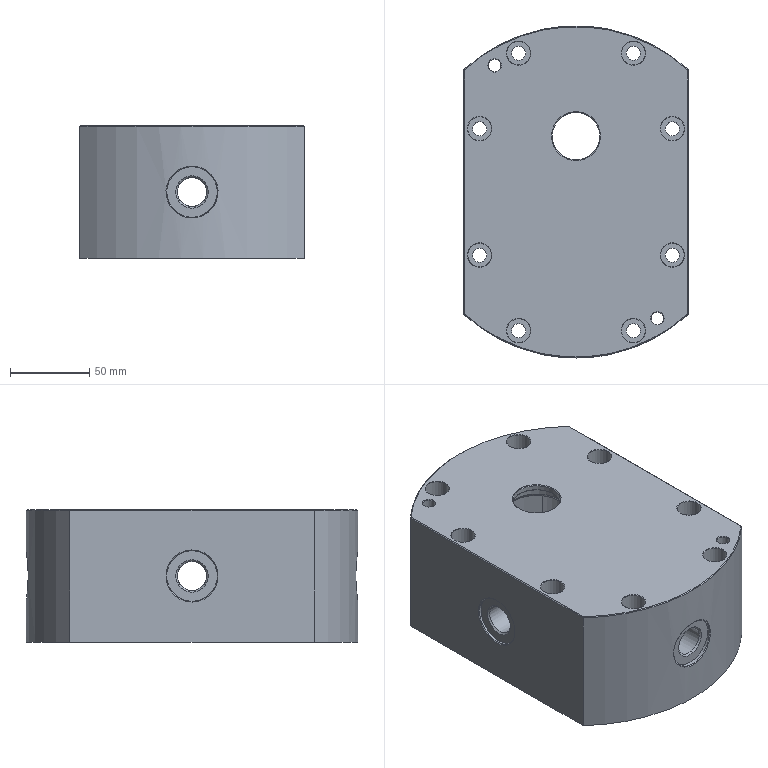Part | 1 solid | 99 faces | box 142 x 210 x 84 mm | volume 1074636 mm3 | cylinder 48 | plane 28 | cone 21 | spline 2 | commonest cylinder face diameters 9 x8 15 x8 30 x5 18.5 x4 32 x4 36 x4